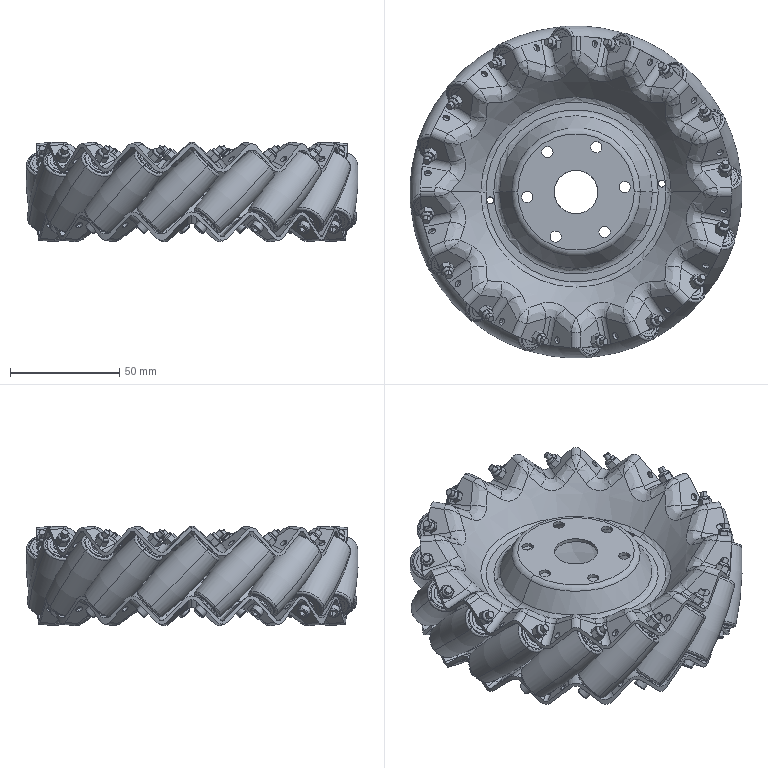Part | SolidWorks | features BaseBody 146 | 146 solids | 2134 faces | box 152.394 x 152.394 x 45.547 mm | volume 219061 mm3 | cylinder 932 | plane 696 | spline 286 | torus 140 | cone 80 | commonest cylinder face diameters 3 x160 5 x128 10 x128 3.2 x116 6.35 x78 7 x64